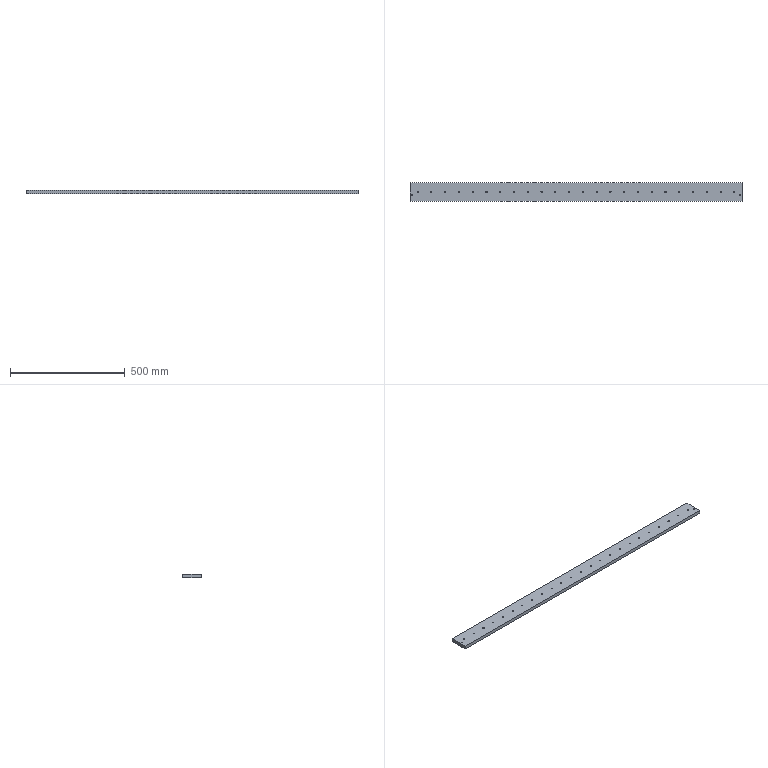Part | NX | 1 solid | 36 faces | box 1446 x 80 x 15 mm | volume 1727896 mm3 | cylinder 26 | plane 6 | cone 4 | commonest cylinder face diameters 5 x24 3 x2
STEP:
#1=CARTESIAN_POINT('',(723.,-40.,0.));
#2=VERTEX_POINT('',#1);
#3=CARTESIAN_POINT('',(723.,40.,0.));
#4=VERTEX_POINT('',#3);
#5=CARTESIAN_POINT('',(723.,-40.,0.));
#6=DIRECTION('',(0.,1.,0.));
#7=VECTOR('',#6,1000.);
#8=LINE('',#5,#7);
#9=EDGE_CURVE('',#2,#4,#8,.T.);
#10=ORIENTED_EDGE('',*,*,#9,.T.);
#11=CARTESIAN_POINT('',(723.,40.,15.));
#12=VERTEX_POINT('',#11);
#13=CARTESIAN_POINT('',(723.,40.,15.));
#14=DIRECTION('',(0.,0.,-1.));
#15=VECTOR('',#14,1000.);
#16=LINE('',#13,#15);
#17=EDGE_CURVE('',#12,#4,#16,.T.);
#18=ORIENTED_EDGE('',*,*,#17,.F.);
#19=CARTESIAN_POINT('',(723.,-40.,15.));
#20=VERTEX_POINT('',#19);
#21=CARTESIAN_POINT('',(723.,-40.,15.));
#22=DIRECTION('',(0.,1.,0.));
#23=VECTOR('',#22,1000.);
#24=LINE('',#21,#23);
#25=EDGE_CURVE('',#20,#12,#24,.T.);
#26=ORIENTED_EDGE('',*,*,#25,.F.);
#27=CARTESIAN_POINT('',(723.,-40.,15.));
#28=DIRECTION('',(0.,0.,-1.));
#29=VECTOR('',#28,1000.);
#30=LINE('',#27,#29);
#31=EDGE_CURVE('',#20,#2,#30,.T.);
#32=ORIENTED_EDGE('',*,*,#31,.T.);
#33=EDGE_LOOP('',(#10,#18,#26,#32));
#34=FACE_BOUND('',#33,.T.);
#35=CARTESIAN_POINT('',(723.,-40.,15.));
#36=DIRECTION('',(-1.,0.,0.));
#37=DIRECTION('',(0.,0.,1.));
#38=AXIS2_PLACEMENT_3D('',#35,#36,#37);
#39=PLANE('',#38);
#40=ADVANCED_FACE('',(#34),#39,.F.);
#41=CARTESIAN_POINT('',(-723.,40.,0.));
#42=VERTEX_POINT('',#41);
#43=CARTESIAN_POINT('',(-723.,40.,0.));
#44=DIRECTION('',(-1.,0.,0.));
#45=VECTOR('',#44,1000.);
#46=LINE('',#43,#45);
#47=EDGE_CURVE('',#4,#42,#46,.T.);
#48=ORIENTED_EDGE('',*,*,#47,.T.);
#49=CARTESIAN_POINT('',(-723.,40.,15.));
#50=VERTEX_POINT('',#49);
#51=CARTESIAN_POINT('',(-723.,40.,15.));
#52=DIRECTION('',(0.,0.,-1.));
#53=VECTOR('',#52,1000.);
#54=LINE('',#51,#53);
#55=EDGE_CURVE('',#50,#42,#54,.T.);
#56=ORIENTED_EDGE('',*,*,#55,.F.);
#57=CARTESIAN_POINT('',(-723.,40.,15.));
#58=DIRECTION('',(-1.,0.,0.));
#59=VECTOR('',#58,1000.);
#60=LINE('',#57,#59);
#61=EDGE_CURVE('',#12,#50,#60,.T.);
#62=ORIENTED_EDGE('',*,*,#61,.F.);
#63=ORIENTED_EDGE('',*,*,#17,.T.);
#64=EDGE_LOOP('',(#48,#56,#62,#63));
#65=FACE_BOUND('',#64,.T.);
#66=CARTESIAN_POINT('',(-723.,40.,15.));
#67=DIRECTION('',(0.,-1.,0.));
#68=DIRECTION('',(0.,0.,-1.));
#69=AXIS2_PLACEMENT_3D('',#66,#67,#68);
#70=PLANE('',#69);
#71=ADVANCED_FACE('',(#65),#70,.F.);
#72=CARTESIAN_POINT('',(-723.,-40.,0.));
#73=VERTEX_POINT('',#72);
#74=CARTESIAN_POINT('',(-723.,-40.,0.));
#75=DIRECTION('',(0.,-1.,0.));
#76=VECTOR('',#75,1000.);
#77=LINE('',#74,#76);
#78=EDGE_CURVE('',#42,#73,#77,.T.);
#79=ORIENTED_EDGE('',*,*,#78,.T.);
#80=CARTESIAN_POINT('',(-723.,-40.,15.));
#81=VERTEX_POINT('',#80);
#82=CARTESIAN_POINT('',(-723.,-40.,15.));
#83=DIRECTION('',(0.,0.,-1.));
#84=VECTOR('',#83,1000.);
#85=LINE('',#82,#84);
#86=EDGE_CURVE('',#81,#73,#85,.T.);
#87=ORIENTED_EDGE('',*,*,#86,.F.);
#88=CARTESIAN_POINT('',(-723.,-40.,15.));
#89=DIRECTION('',(0.,-1.,0.));
#90=VECTOR('',#89,1000.);
#91=LINE('',#88,#90);
#92=EDGE_CURVE('',#50,#81,#91,.T.);
#93=ORIENTED_EDGE('',*,*,#92,.F.);
#94=ORIENTED_EDGE('',*,*,#55,.T.);
#95=EDGE_LOOP('',(#79,#87,#93,#94));
#96=FACE_BOUND('',#95,.T.);
#97=CARTESIAN_POINT('',(-723.,-40.,15.));
#98=DIRECTION('',(1.,0.,0.));
#99=DIRECTION('',(0.,0.,-1.));
#100=AXIS2_PLACEMENT_3D('',#97,#98,#99);
#101=PLANE('',#100);
#102=ADVANCED_FACE('',(#96),#101,.F.);
#103=CARTESIAN_POINT('',(-723.,-40.,0.));
#104=DIRECTION('',(1.,0.,0.));
#105=VECTOR('',#104,1000.);
#106=LINE('',#103,#105);
#107=EDGE_CURVE('',#73,#2,#106,.T.);
#108=ORIENTED_EDGE('',*,*,#107,.T.);
#109=ORIENTED_EDGE('',*,*,#31,.F.);
#110=CARTESIAN_POINT('',(-723.,-40.,15.));
#111=DIRECTION('',(1.,0.,0.));
#112=VECTOR('',#111,1000.);
#113=LINE('',#110,#112);
#114=EDGE_CURVE('',#81,#20,#113,.T.);
#115=ORIENTED_EDGE('',*,*,#114,.F.);
#116=ORIENTED_EDGE('',*,*,#86,.T.);
#117=EDGE_LOOP('',(#108,#109,#115,#116));
#118=FACE_BOUND('',#117,.T.);
#119=CARTESIAN_POINT('',(-723.,-40.,15.));
#120=DIRECTION('',(0.,1.,0.));
#121=DIRECTION('',(0.,0.,1.));
#122=AXIS2_PLACEMENT_3D('',#119,#120,#121);
#123=PLANE('',#122);
#124=ADVANCED_FACE('',(#118),#123,.F.);
#125=CARTESIAN_POINT('',(710.5,-13.,15.));
#126=VERTEX_POINT('',#125);
#127=CARTESIAN_POINT('',(713.,-13.,15.));
#128=DIRECTION('',(0.,0.,-1.));
#129=DIRECTION('',(-1.,0.,0.));
#130=AXIS2_PLACEMENT_3D('',#127,#128,#129);
#131=CIRCLE('',#130,2.5);
#132=EDGE_CURVE('',#126,#126,#131,.T.);
#133=ORIENTED_EDGE('',*,*,#132,.T.);
#134=EDGE_LOOP('',(#133));
#135=FACE_BOUND('',#134,.T.);
#136=CARTESIAN_POINT('',(-715.5,-13.,15.));
#137=VERTEX_POINT('',#136);
#138=CARTESIAN_POINT('',(-713.,-13.,15.));
#139=DIRECTION('',(0.,0.,-1.));
#140=DIRECTION('',(-1.,0.,0.));
#141=AXIS2_PLACEMENT_3D('',#138,#139,#140);
#142=CIRCLE('',#141,2.5);
#143=EDGE_CURVE('',#137,#137,#142,.T.);
#144=ORIENTED_EDGE('',*,*,#143,.T.);
#145=EDGE_LOOP('',(#144));
#146=FACE_BOUND('',#145,.T.);
#147=CARTESIAN_POINT('',(-627.5,0.,15.));
#148=VERTEX_POINT('',#147);
#149=CARTESIAN_POINT('',(-630.,0.,15.));
#150=DIRECTION('',(0.,0.,1.));
#151=DIRECTION('',(1.,0.,0.));
#152=AXIS2_PLACEMENT_3D('',#149,#150,#151);
#153=CIRCLE('',#152,2.5);
#154=EDGE_CURVE('',#148,#148,#153,.T.);
#155=ORIENTED_EDGE('',*,*,#154,.F.);
#156=EDGE_LOOP('',(#155));
#157=FACE_BOUND('',#156,.T.);
#158=CARTESIAN_POINT('',(-687.5,0.,15.));
#159=VERTEX_POINT('',#158);
#160=CARTESIAN_POINT('',(-690.,0.,15.));
#161=DIRECTION('',(0.,0.,1.));
#162=DIRECTION('',(1.,0.,0.));
#163=AXIS2_PLACEMENT_3D('',#160,#161,#162);
#164=CIRCLE('',#163,2.5);
#165=EDGE_CURVE('',#159,#159,#164,.T.);
#166=ORIENTED_EDGE('',*,*,#165,.F.);
#167=EDGE_LOOP('',(#166));
#168=FACE_BOUND('',#167,.T.);
#169=ORIENTED_EDGE('',*,*,#25,.T.);
#170=ORIENTED_EDGE('',*,*,#61,.T.);
#171=ORIENTED_EDGE('',*,*,#92,.T.);
#172=ORIENTED_EDGE('',*,*,#114,.T.);
#173=EDGE_LOOP('',(#169,#170,#171,#172));
#174=FACE_BOUND('',#173,.T.);
#175=CARTESIAN_POINT('',(-567.5,0.,15.));
#176=VERTEX_POINT('',#175);
#177=CARTESIAN_POINT('',(-570.,0.,15.));
#178=DIRECTION('',(0.,0.,1.));
#179=DIRECTION('',(1.,0.,0.));
#180=AXIS2_PLACEMENT_3D('',#177,#178,#179);
#181=CIRCLE('',#180,2.5);
#182=EDGE_CURVE('',#176,#176,#181,.T.);
#183=ORIENTED_EDGE('',*,*,#182,.F.);
#184=EDGE_LOOP('',(#183));
#185=FACE_BOUND('',#184,.T.);
#186=CARTESIAN_POINT('',(-507.5,0.,15.));
#187=VERTEX_POINT('',#186);
#188=CARTESIAN_POINT('',(-510.,0.,15.));
#189=DIRECTION('',(0.,0.,1.));
#190=DIRECTION('',(1.,0.,0.));
#191=AXIS2_PLACEMENT_3D('',#188,#189,#190);
#192=CIRCLE('',#191,2.5);
#193=EDGE_CURVE('',#187,#187,#192,.T.);
#194=ORIENTED_EDGE('',*,*,#193,.F.);
#195=EDGE_LOOP('',(#194));
#196=FACE_BOUND('',#195,.T.);
#197=CARTESIAN_POINT('',(-447.5,0.,15.));
#198=VERTEX_POINT('',#197);
#199=CARTESIAN_POINT('',(-450.,0.,15.));
#200=DIRECTION('',(0.,0.,1.));
#201=DIRECTION('',(1.,0.,0.));
#202=AXIS2_PLACEMENT_3D('',#199,#200,#201);
#203=CIRCLE('',#202,2.5);
#204=EDGE_CURVE('',#198,#198,#203,.T.);
#205=ORIENTED_EDGE('',*,*,#204,.F.);
#206=EDGE_LOOP('',(#205));
#207=FACE_BOUND('',#206,.T.);
#208=CARTESIAN_POINT('',(-387.5,0.,15.));
#209=VERTEX_POINT('',#208);
#210=CARTESIAN_POINT('',(-390.,0.,15.));
#211=DIRECTION('',(0.,0.,1.));
#212=DIRECTION('',(1.,0.,0.));
#213=AXIS2_PLACEMENT_3D('',#210,#211,#212);
#214=CIRCLE('',#213,2.5);
#215=EDGE_CURVE('',#209,#209,#214,.T.);
#216=ORIENTED_EDGE('',*,*,#215,.F.);
#217=EDGE_LOOP('',(#216));
#218=FACE_BOUND('',#217,.T.);
#219=CARTESIAN_POINT('',(-327.5,0.,15.));
#220=VERTEX_POINT('',#219);
#221=CARTESIAN_POINT('',(-330.,0.,15.));
#222=DIRECTION('',(0.,0.,1.));
#223=DIRECTION('',(1.,0.,0.));
#224=AXIS2_PLACEMENT_3D('',#221,#222,#223);
#225=CIRCLE('',#224,2.5);
#226=EDGE_CURVE('',#220,#220,#225,.T.);
#227=ORIENTED_EDGE('',*,*,#226,.F.);
#228=EDGE_LOOP('',(#227));
#229=FACE_BOUND('',#228,.T.);
#230=CARTESIAN_POINT('',(-267.5,0.,15.));
#231=VERTEX_POINT('',#230);
#232=CARTESIAN_POINT('',(-270.,0.,15.));
#233=DIRECTION('',(0.,0.,1.));
#234=DIRECTION('',(1.,0.,0.));
#235=AXIS2_PLACEMENT_3D('',#232,#233,#234);
#236=CIRCLE('',#235,2.5);
#237=EDGE_CURVE('',#231,#231,#236,.T.);
#238=ORIENTED_EDGE('',*,*,#237,.F.);
#239=EDGE_LOOP('',(#238));
#240=FACE_BOUND('',#239,.T.);
#241=CARTESIAN_POINT('',(-207.5,0.,15.));
#242=VERTEX_POINT('',#241);
#243=CARTESIAN_POINT('',(-210.,0.,15.));
#244=DIRECTION('',(0.,0.,1.));
#245=DIRECTION('',(1.,0.,0.));
#246=AXIS2_PLACEMENT_3D('',#243,#244,#245);
#247=CIRCLE('',#246,2.5);
#248=EDGE_CURVE('',#242,#242,#247,.T.);
#249=ORIENTED_EDGE('',*,*,#248,.F.);
#250=EDGE_LOOP('',(#249));
#251=FACE_BOUND('',#250,.T.);
#252=CARTESIAN_POINT('',(-147.5,0.,15.));
#253=VERTEX_POINT('',#252);
#254=CARTESIAN_POINT('',(-150.,0.,15.));
#255=DIRECTION('',(0.,0.,1.));
#256=DIRECTION('',(1.,0.,0.));
#257=AXIS2_PLACEMENT_3D('',#254,#255,#256);
#258=CIRCLE('',#257,2.5);
#259=EDGE_CURVE('',#253,#253,#258,.T.);
#260=ORIENTED_EDGE('',*,*,#259,.F.);
#261=EDGE_LOOP('',(#260));
#262=FACE_BOUND('',#261,.T.);
#263=CARTESIAN_POINT('',(-87.5,0.,15.));
#264=VERTEX_POINT('',#263);
#265=CARTESIAN_POINT('',(-90.,0.,15.));
#266=DIRECTION('',(0.,0.,1.));
#267=DIRECTION('',(1.,0.,0.));
#268=AXIS2_PLACEMENT_3D('',#265,#266,#267);
#269=CIRCLE('',#268,2.5);
#270=EDGE_CURVE('',#264,#264,#269,.T.);
#271=ORIENTED_EDGE('',*,*,#270,.F.);
#272=EDGE_LOOP('',(#271));
#273=FACE_BOUND('',#272,.T.);
#274=CARTESIAN_POINT('',(-27.5,0.,15.));
#275=VERTEX_POINT('',#274);
#276=CARTESIAN_POINT('',(-30.,0.,15.));
#277=DIRECTION('',(0.,0.,1.));
#278=DIRECTION('',(1.,0.,0.));
#279=AXIS2_PLACEMENT_3D('',#276,#277,#278);
#280=CIRCLE('',#279,2.5);
#281=EDGE_CURVE('',#275,#275,#280,.T.);
#282=ORIENTED_EDGE('',*,*,#281,.F.);
#283=EDGE_LOOP('',(#282));
#284=FACE_BOUND('',#283,.T.);
#285=CARTESIAN_POINT('',(32.5,0.,15.));
#286=VERTEX_POINT('',#285);
#287=CARTESIAN_POINT('',(30.,0.,15.));
#288=DIRECTION('',(0.,0.,1.));
#289=DIRECTION('',(1.,0.,0.));
#290=AXIS2_PLACEMENT_3D('',#287,#288,#289);
#291=CIRCLE('',#290,2.5);
#292=EDGE_CURVE('',#286,#286,#291,.T.);
#293=ORIENTED_EDGE('',*,*,#292,.F.);
#294=EDGE_LOOP('',(#293));
#295=FACE_BOUND('',#294,.T.);
#296=CARTESIAN_POINT('',(92.5,0.,15.));
#297=VERTEX_POINT('',#296);
#298=CARTESIAN_POINT('',(90.,0.,15.));
#299=DIRECTION('',(0.,0.,1.));
#300=DIRECTION('',(1.,0.,0.));
#301=AXIS2_PLACEMENT_3D('',#298,#299,#300);
#302=CIRCLE('',#301,2.5);
#303=EDGE_CURVE('',#297,#297,#302,.T.);
#304=ORIENTED_EDGE('',*,*,#303,.F.);
#305=EDGE_LOOP('',(#304));
#306=FACE_BOUND('',#305,.T.);
#307=CARTESIAN_POINT('',(152.5,0.,15.));
#308=VERTEX_POINT('',#307);
#309=CARTESIAN_POINT('',(150.,0.,15.));
#310=DIRECTION('',(0.,0.,1.));
#311=DIRECTION('',(1.,0.,0.));
#312=AXIS2_PLACEMENT_3D('',#309,#310,#311);
#313=CIRCLE('',#312,2.5);
#314=EDGE_CURVE('',#308,#308,#313,.T.);
#315=ORIENTED_EDGE('',*,*,#314,.F.);
#316=EDGE_LOOP('',(#315));
#317=FACE_BOUND('',#316,.T.);
#318=CARTESIAN_POINT('',(212.5,0.,15.));
#319=VERTEX_POINT('',#318);
#320=CARTESIAN_POINT('',(210.,0.,15.));
#321=DIRECTION('',(0.,0.,1.));
#322=DIRECTION('',(1.,0.,0.));
#323=AXIS2_PLACEMENT_3D('',#320,#321,#322);
#324=CIRCLE('',#323,2.5);
#325=EDGE_CURVE('',#319,#319,#324,.T.);
#326=ORIENTED_EDGE('',*,*,#325,.F.);
#327=EDGE_LOOP('',(#326));
#328=FACE_BOUND('',#327,.T.);
#329=CARTESIAN_POINT('',(272.5,0.,15.));
#330=VERTEX_POINT('',#329);
#331=CARTESIAN_POINT('',(270.,0.,15.));
#332=DIRECTION('',(0.,0.,1.));
#333=DIRECTION('',(1.,0.,0.));
#334=AXIS2_PLACEMENT_3D('',#331,#332,#333);
#335=CIRCLE('',#334,2.5);
#336=EDGE_CURVE('',#330,#330,#335,.T.);
#337=ORIENTED_EDGE('',*,*,#336,.F.);
#338=EDGE_LOOP('',(#337));
#339=FACE_BOUND('',#338,.T.);
#340=CARTESIAN_POINT('',(332.5,0.,15.));
#341=VERTEX_POINT('',#340);
#342=CARTESIAN_POINT('',(330.,0.,15.));
#343=DIRECTION('',(0.,0.,1.));
#344=DIRECTION('',(1.,0.,0.));
#345=AXIS2_PLACEMENT_3D('',#342,#343,#344);
#346=CIRCLE('',#345,2.5);
#347=EDGE_CURVE('',#341,#341,#346,.T.);
#348=ORIENTED_EDGE('',*,*,#347,.F.);
#349=EDGE_LOOP('',(#348));
#350=FACE_BOUND('',#349,.T.);
#351=CARTESIAN_POINT('',(392.5,0.,15.));
#352=VERTEX_POINT('',#351);
#353=CARTESIAN_POINT('',(390.,0.,15.));
#354=DIRECTION('',(0.,0.,1.));
#355=DIRECTION('',(1.,0.,0.));
#356=AXIS2_PLACEMENT_3D('',#353,#354,#355);
#357=CIRCLE('',#356,2.5);
#358=EDGE_CURVE('',#352,#352,#357,.T.);
#359=ORIENTED_EDGE('',*,*,#358,.F.);
#360=EDGE_LOOP('',(#359));
#361=FACE_BOUND('',#360,.T.);
#362=CARTESIAN_POINT('',(452.5,0.,15.));
#363=VERTEX_POINT('',#362);
#364=CARTESIAN_POINT('',(450.,0.,15.));
#365=DIRECTION('',(0.,0.,1.));
#366=DIRECTION('',(1.,0.,0.));
#367=AXIS2_PLACEMENT_3D('',#364,#365,#366);
#368=CIRCLE('',#367,2.5);
#369=EDGE_CURVE('',#363,#363,#368,.T.);
#370=ORIENTED_EDGE('',*,*,#369,.F.);
#371=EDGE_LOOP('',(#370));
#372=FACE_BOUND('',#371,.T.);
#373=CARTESIAN_POINT('',(512.5,0.,15.));
#374=VERTEX_POINT('',#373);
#375=CARTESIAN_POINT('',(510.,0.,15.));
#376=DIRECTION('',(0.,0.,1.));
#377=DIRECTION('',(1.,0.,0.));
#378=AXIS2_PLACEMENT_3D('',#375,#376,#377);
#379=CIRCLE('',#378,2.5);
#380=EDGE_CURVE('',#374,#374,#379,.T.);
#381=ORIENTED_EDGE('',*,*,#380,.F.);
#382=EDGE_LOOP('',(#381));
#383=FACE_BOUND('',#382,.T.);
#384=CARTESIAN_POINT('',(572.5,0.,15.));
#385=VERTEX_POINT('',#384);
#386=CARTESIAN_POINT('',(570.,0.,15.));
#387=DIRECTION('',(0.,0.,1.));
#388=DIRECTION('',(1.,0.,0.));
#389=AXIS2_PLACEMENT_3D('',#386,#387,#388);
#390=CIRCLE('',#389,2.5);
#391=EDGE_CURVE('',#385,#385,#390,.T.);
#392=ORIENTED_EDGE('',*,*,#391,.F.);
#393=EDGE_LOOP('',(#392));
#394=FACE_BOUND('',#393,.T.);
#395=CARTESIAN_POINT('',(632.5,0.,15.));
#396=VERTEX_POINT('',#395);
#397=CARTESIAN_POINT('',(630.,0.,15.));
#398=DIRECTION('',(0.,0.,1.));
#399=DIRECTION('',(1.,0.,0.));
#400=AXIS2_PLACEMENT_3D('',#397,#398,#399);
#401=CIRCLE('',#400,2.5);
#402=EDGE_CURVE('',#396,#396,#401,.T.);
#403=ORIENTED_EDGE('',*,*,#402,.F.);
#404=EDGE_LOOP('',(#403));
#405=FACE_BOUND('',#404,.T.);
#406=CARTESIAN_POINT('',(692.5,0.,15.));
#407=VERTEX_POINT('',#406);
#408=CARTESIAN_POINT('',(690.,0.,15.));
#409=DIRECTION('',(0.,0.,1.));
#410=DIRECTION('',(1.,0.,0.));
#411=AXIS2_PLACEMENT_3D('',#408,#409,#410);
#412=CIRCLE('',#411,2.5);
#413=EDGE_CURVE('',#407,#407,#412,.T.);
#414=ORIENTED_EDGE('',*,*,#413,.F.);
#415=EDGE_LOOP('',(#414));
#416=FACE_BOUND('',#415,.T.);
#417=CARTESIAN_POINT('',(0.,0.,15.));
#418=DIRECTION('',(0.,0.,-1.));
#419=DIRECTION('',(-1.,0.,0.));
#420=AXIS2_PLACEMENT_3D('',#417,#418,#419);
#421=PLANE('',#420);
#422=ADVANCED_FACE('',(#135,#146,#157,#168,#174,#185,#196,#207,#218,#229,#240,#251,#262,#273,#284,#295,#306,#317,#328,#339,#350,#361,#372,#383,#394,#405,#416),#421,.F.);
#423=CARTESIAN_POINT('',(710.5,-13.,0.));
#424=VERTEX_POINT('',#423);
#425=CARTESIAN_POINT('',(713.,-13.,0.));
#426=DIRECTION('',(0.,0.,-1.));
#427=DIRECTION('',(-1.,0.,0.));
#428=AXIS2_PLACEMENT_3D('',#425,#426,#427);
#429=CIRCLE('',#428,2.5);
#430=EDGE_CURVE('',#424,#424,#429,.F.);
#431=ORIENTED_EDGE('',*,*,#430,.T.);
#432=EDGE_LOOP('',(#431));
#433=FACE_BOUND('',#432,.T.);
#434=CARTESIAN_POINT('',(-715.5,-13.,0.));
#435=VERTEX_POINT('',#434);
#436=CARTESIAN_POINT('',(-713.,-13.,0.));
#437=DIRECTION('',(0.,0.,-1.));
#438=DIRECTION('',(-1.,0.,0.));
#439=AXIS2_PLACEMENT_3D('',#436,#437,#438);
#440=CIRCLE('',#439,2.5);
#441=EDGE_CURVE('',#435,#435,#440,.F.);
#442=ORIENTED_EDGE('',*,*,#441,.T.);
#443=EDGE_LOOP('',(#442));
#444=FACE_BOUND('',#443,.T.);
#445=CARTESIAN_POINT('',(-632.5,0.,0.));
#446=VERTEX_POINT('',#445);
#447=CARTESIAN_POINT('',(-630.,0.,0.));
#448=DIRECTION('',(0.,0.,-1.));
#449=DIRECTION('',(-1.,0.,0.));
#450=AXIS2_PLACEMENT_3D('',#447,#448,#449);
#451=CIRCLE('',#450,2.5);
#452=EDGE_CURVE('',#446,#446,#451,.T.);
#453=ORIENTED_EDGE('',*,*,#452,.F.);
#454=EDGE_LOOP('',(#453));
#455=FACE_BOUND('',#454,.T.);
#456=CARTESIAN_POINT('',(-692.5,0.,0.));
#457=VERTEX_POINT('',#456);
#458=CARTESIAN_POINT('',(-690.,0.,0.));
#459=DIRECTION('',(0.,0.,-1.));
#460=DIRECTION('',(-1.,0.,0.));
#461=AXIS2_PLACEMENT_3D('',#458,#459,#460);
#462=CIRCLE('',#461,2.5);
#463=EDGE_CURVE('',#457,#457,#462,.T.);
#464=ORIENTED_EDGE('',*,*,#463,.F.);
#465=EDGE_LOOP('',(#464));
#466=FACE_BOUND('',#465,.T.);
#467=ORIENTED_EDGE('',*,*,#9,.F.);
#468=ORIENTED_EDGE('',*,*,#107,.F.);
#469=ORIENTED_EDGE('',*,*,#78,.F.);
#470=ORIENTED_EDGE('',*,*,#47,.F.);
#471=EDGE_LOOP('',(#467,#468,#469,#470));
#472=FACE_BOUND('',#471,.T.);
#473=CARTESIAN_POINT('',(-572.5,0.,0.));
#474=VERTEX_POINT('',#473);
#475=CARTESIAN_POINT('',(-570.,0.,0.));
#476=DIRECTION('',(0.,0.,-1.));
#477=DIRECTION('',(-1.,0.,0.));
#478=AXIS2_PLACEMENT_3D('',#475,#476,#477);
#479=CIRCLE('',#478,2.5);
#480=EDGE_CURVE('',#474,#474,#479,.T.);
#481=ORIENTED_EDGE('',*,*,#480,.F.);
#482=EDGE_LOOP('',(#481));
#483=FACE_BOUND('',#482,.T.);
#484=CARTESIAN_POINT('',(-512.5,0.,0.));
#485=VERTEX_POINT('',#484);
#486=CARTESIAN_POINT('',(-510.,0.,0.));
#487=DIRECTION('',(0.,0.,-1.));
#488=DIRECTION('',(-1.,0.,0.));
#489=AXIS2_PLACEMENT_3D('',#486,#487,#488);
#490=CIRCLE('',#489,2.5);
#491=EDGE_CURVE('',#485,#485,#490,.T.);
#492=ORIENTED_EDGE('',*,*,#491,.F.);
#493=EDGE_LOOP('',(#492));
#494=FACE_BOUND('',#493,.T.);
#495=CARTESIAN_POINT('',(-452.5,0.,0.));
#496=VERTEX_POINT('',#495);
#497=CARTESIAN_POINT('',(-450.,0.,0.));
#498=DIRECTION('',(0.,0.,-1.));
#499=DIRECTION('',(-1.,0.,0.));
#500=AXIS2_PLACEMENT_3D('',#497,#498,#499);
#501=CIRCLE('',#500,2.5);
#502=EDGE_CURVE('',#496,#496,#501,.T.);
#503=ORIENTED_EDGE('',*,*,#502,.F.);
#504=EDGE_LOOP('',(#503));
#505=FACE_BOUND('',#504,.T.);
#506=CARTESIAN_POINT('',(-392.5,0.,0.));
#507=VERTEX_POINT('',#506);
#508=CARTESIAN_POINT('',(-390.,0.,0.));
#509=DIRECTION('',(0.,0.,-1.));
#510=DIRECTION('',(-1.,0.,0.));
#511=AXIS2_PLACEMENT_3D('',#508,#509,#510);
#512=CIRCLE('',#511,2.5);
#513=EDGE_CURVE('',#507,#507,#512,.T.);
#514=ORIENTED_EDGE('',*,*,#513,.F.);
#515=EDGE_LOOP('',(#514));
#516=FACE_BOUND('',#515,.T.);
#517=CARTESIAN_POINT('',(-332.5,0.,0.));
#518=VERTEX_POINT('',#517);
#519=CARTESIAN_POINT('',(-330.,0.,0.));
#520=DIRECTION('',(0.,0.,-1.));
#521=DIRECTION('',(-1.,0.,0.));
#522=AXIS2_PLACEMENT_3D('',#519,#520,#521);
#523=CIRCLE('',#522,2.5);
#524=EDGE_CURVE('',#518,#518,#523,.T.);
#525=ORIENTED_EDGE('',*,*,#524,.F.);
#526=EDGE_LOOP('',(#525));
#527=FACE_BOUND('',#526,.T.);
#528=CARTESIAN_POINT('',(-272.5,0.,0.));
#529=VERTEX_POINT('',#528);
#530=CARTESIAN_POINT('',(-270.,0.,0.));
#531=DIRECTION('',(0.,0.,-1.));
#532=DIRECTION('',(-1.,0.,0.));
#533=AXIS2_PLACEMENT_3D('',#530,#531,#532);
#534=CIRCLE('',#533,2.5);
#535=EDGE_CURVE('',#529,#529,#534,.T.);
#536=ORIENTED_EDGE('',*,*,#535,.F.);
#537=EDGE_LOOP('',(#536));
#538=FACE_BOUND('',#537,.T.);
#539=CARTESIAN_POINT('',(-212.5,0.,0.));
#540=VERTEX_POINT('',#539);
#541=CARTESIAN_POINT('',(-210.,0.,0.));
#542=DIRECTION('',(0.,0.,-1.));
#543=DIRECTION('',(-1.,0.,0.));
#544=AXIS2_PLACEMENT_3D('',#541,#542,#543);
#545=CIRCLE('',#544,2.5);
#546=EDGE_CURVE('',#540,#540,#545,.T.);
#547=ORIENTED_EDGE('',*,*,#546,.F.);
#548=EDGE_LOOP('',(#547));
#549=FACE_BOUND('',#548,.T.);
#550=CARTESIAN_POINT('',(-152.5,0.,0.));
#551=VERTEX_POINT('',#550);
#552=CARTESIAN_POINT('',(-150.,0.,0.));
#553=DIRECTION('',(0.,0.,-1.));
#554=DIRECTION('',(-1.,0.,0.));
#555=AXIS2_PLACEMENT_3D('',#552,#553,#554);
#556=CIRCLE('',#555,2.5);
#557=EDGE_CURVE('',#551,#551,#556,.T.);
#558=ORIENTED_EDGE('',*,*,#557,.F.);
#559=EDGE_LOOP('',(#558));
#560=FACE_BOUND('',#559,.T.);
#561=CARTESIAN_POINT('',(-92.5,0.,0.));
#562=VERTEX_POINT('',#561);
#563=CARTESIAN_POINT('',(-90.,0.,0.));
#564=DIRECTION('',(0.,0.,-1.));
#565=DIRECTION('',(-1.,0.,0.));
#566=AXIS2_PLACEMENT_3D('',#563,#564,#565);
#567=CIRCLE('',#566,2.5);
#568=EDGE_CURVE('',#562,#562,#567,.T.);
#569=ORIENTED_EDGE('',*,*,#568,.F.);
#570=EDGE_LOOP('',(#569));
#571=FACE_BOUND('',#570,.T.);
#572=CARTESIAN_POINT('',(-32.5,0.,0.));
#573=VERTEX_POINT('',#572);
#574=CARTESIAN_POINT('',(-30.,0.,0.));
#575=DIRECTION('',(0.,0.,-1.));
#576=DIRECTION('',(-1.,0.,0.));
#577=AXIS2_PLACEMENT_3D('',#574,#575,#576);
#578=CIRCLE('',#577,2.5);
#579=EDGE_CURVE('',#573,#573,#578,.T.);
#580=ORIENTED_EDGE('',*,*,#579,.F.);
#581=EDGE_LOOP('',(#580));
#582=FACE_BOUND('',#581,.T.);
#583=CARTESIAN_POINT('',(27.5,0.,0.));
#584=VERTEX_POINT('',#583);
#585=CARTESIAN_POINT('',(30.,0.,0.));
#586=DIRECTION('',(0.,0.,-1.));
#587=DIRECTION('',(-1.,0.,0.));
#588=AXIS2_PLACEMENT_3D('',#585,#586,#587);
#589=CIRCLE('',#588,2.5);
#590=EDGE_CURVE('',#584,#584,#589,.T.);
#591=ORIENTED_EDGE('',*,*,#590,.F.);
#592=EDGE_LOOP('',(#591));
#593=FACE_BOUND('',#592,.T.);
#594=CARTESIAN_POINT('',(87.5,0.,0.));
#595=VERTEX_POINT('',#594);
#596=CARTESIAN_POINT('',(90.,0.,0.));
#597=DIRECTION('',(0.,0.,-1.));
#598=DIRECTION('',(-1.,0.,0.));
#599=AXIS2_PLACEMENT_3D('',#596,#597,#598);
#600=CIRCLE('',#599,2.5);
#601=EDGE_CURVE('',#595,#595,#600,.T.);
#602=ORIENTED_EDGE('',*,*,#601,.F.);
#603=EDGE_LOOP('',(#602));
#604=FACE_BOUND('',#603,.T.);
#605=CARTESIAN_POINT('',(147.5,0.,0.));
#606=VERTEX_POINT('',#605);
#607=CARTESIAN_POINT('',(150.,0.,0.));
#608=DIRECTION('',(0.,0.,-1.));
#609=DIRECTION('',(-1.,0.,0.));
#610=AXIS2_PLACEMENT_3D('',#607,#608,#609);
#611=CIRCLE('',#610,2.5);
#612=EDGE_CURVE('',#606,#606,#611,.T.);
#613=ORIENTED_EDGE('',*,*,#612,.F.);
#614=EDGE_LOOP('',(#613));
#615=FACE_BOUND('',#614,.T.);
#616=CARTESIAN_POINT('',(207.5,0.,0.));
#617=VERTEX_POINT('',#616);
#618=CARTESIAN_POINT('',(210.,0.,0.));
#619=DIRECTION('',(0.,0.,-1.));
#620=DIRECTION('',(-1.,0.,0.));
#621=AXIS2_PLACEMENT_3D('',#618,#619,#620);
#622=CIRCLE('',#621,2.5);
#623=EDGE_CURVE('',#617,#617,#622,.T.);
#624=ORIENTED_EDGE('',*,*,#623,.F.);
#625=EDGE_LOOP('',(#624));
#626=FACE_BOUND('',#625,.T.);
#627=CARTESIAN_POINT('',(267.5,0.,0.));
#628=VERTEX_POINT('',#627);
#629=CARTESIAN_POINT('',(270.,0.,0.));
#630=DIRECTION('',(0.,0.,-1.));
#631=DIRECTION('',(-1.,0.,0.));
#632=AXIS2_PLACEMENT_3D('',#629,#630,#631);
#633=CIRCLE('',#632,2.5);
#634=EDGE_CURVE('',#628,#628,#633,.T.);
#635=ORIENTED_EDGE('',*,*,#634,.F.);
#636=EDGE_LOOP('',(#635));
#637=FACE_BOUND('',#636,.T.);
#638=CARTESIAN_POINT('',(327.5,0.,0.));
#639=VERTEX_POINT('',#638);
#640=CARTESIAN_POINT('',(330.,0.,0.));
#641=DIRECTION('',(0.,0.,-1.));
#642=DIRECTION('',(-1.,0.,0.));
#643=AXIS2_PLACEMENT_3D('',#640,#641,#642);
#644=CIRCLE('',#643,2.5);
#645=EDGE_CURVE('',#639,#639,#644,.T.);
#646=ORIENTED_EDGE('',*,*,#645,.F.);
#647=EDGE_LOOP('',(#646));
#648=FACE_BOUND('',#647,.T.);
#649=CARTESIAN_POINT('',(387.5,0.,0.));
#650=VERTEX_POINT('',#649);
#651=CARTESIAN_POINT('',(390.,0.,0.));
#652=DIRECTION('',(0.,0.,-1.));
#653=DIRECTION('',(-1.,0.,0.));
#654=AXIS2_PLACEMENT_3D('',#651,#652,#653);
#655=CIRCLE('',#654,2.5);
#656=EDGE_CURVE('',#650,#650,#655,.T.);
#657=ORIENTED_EDGE('',*,*,#656,.F.);
#658=EDGE_LOOP('',(#657));
#659=FACE_BOUND('',#658,.T.);
#660=CARTESIAN_POINT('',(447.5,0.,0.));
#661=VERTEX_POINT('',#660);
#662=CARTESIAN_POINT('',(450.,0.,0.));
#663=DIRECTION('',(0.,0.,-1.));
#664=DIRECTION('',(-1.,0.,0.));
#665=AXIS2_PLACEMENT_3D('',#662,#663,#664);
#666=CIRCLE('',#665,2.5);
#667=EDGE_CURVE('',#661,#661,#666,.T.);
#668=ORIENTED_EDGE('',*,*,#667,.F.);
#669=EDGE_LOOP('',(#668));
#670=FACE_BOUND('',#669,.T.);
#671=CARTESIAN_POINT('',(507.5,0.,0.));
#672=VERTEX_POINT('',#671);
#673=CARTESIAN_POINT('',(510.,0.,0.));
#674=DIRECTION('',(0.,0.,-1.));
#675=DIRECTION('',(-1.,0.,0.));
#676=AXIS2_PLACEMENT_3D('',#673,#674,#675);
#677=CIRCLE('',#676,2.5);
#678=EDGE_CURVE('',#672,#672,#677,.T.);
#679=ORIENTED_EDGE('',*,*,#678,.F.);
#680=EDGE_LOOP('',(#679));
#681=FACE_BOUND('',#680,.T.);
#682=CARTESIAN_POINT('',(567.5,0.,0.));
#683=VERTEX_POINT('',#682);
#684=CARTESIAN_POINT('',(570.,0.,0.));
#685=DIRECTION('',(0.,0.,-1.));
#686=DIRECTION('',(-1.,0.,0.));
#687=AXIS2_PLACEMENT_3D('',#684,#685,#686);
#688=CIRCLE('',#687,2.5);
#689=EDGE_CURVE('',#683,#683,#688,.T.);
#690=ORIENTED_EDGE('',*,*,#689,.F.);
#691=EDGE_LOOP('',(#690));
#692=FACE_BOUND('',#691,.T.);
#693=CARTESIAN_POINT('',(627.5,0.,0.));
#694=VERTEX_POINT('',#693);
#695=CARTESIAN_POINT('',(630.,0.,0.));
#696=DIRECTION('',(0.,0.,-1.));
#697=DIRECTION('',(-1.,0.,0.));
#698=AXIS2_PLACEMENT_3D('',#695,#696,#697);
#699=CIRCLE('',#698,2.5);
#700=EDGE_CURVE('',#694,#694,#699,.T.);
#701=ORIENTED_EDGE('',*,*,#700,.F.);
#702=EDGE_LOOP('',(#701));
#703=FACE_BOUND('',#702,.T.);
#704=CARTESIAN_POINT('',(687.5,0.,0.));
#705=VERTEX_POINT('',#704);
#706=CARTESIAN_POINT('',(690.,0.,0.));
#707=DIRECTION('',(0.,0.,-1.));
#708=DIRECTION('',(-1.,0.,0.));
#709=AXIS2_PLACEMENT_3D('',#706,#707,#708);
#710=CIRCLE('',#709,2.5);
#711=EDGE_CURVE('',#705,#705,#710,.T.);
#712=ORIENTED_EDGE('',*,*,#711,.F.);
#713=EDGE_LOOP('',(#712));
#714=FACE_BOUND('',#713,.T.);
#715=CARTESIAN_POINT('',(0.,0.,0.));
#716=DIRECTION('',(0.,0.,-1.));
#717=DIRECTION('',(-1.,0.,0.));
#718=AXIS2_PLACEMENT_3D('',#715,#716,#717);
#719=PLANE('',#718);
#720=ADVANCED_FACE('',(#433,#444,#455,#466,#472,#483,#494,#505,#516,#527,#538,#549,#560,#571,#582,#593,#604,#615,#626,#637,#648,#659,#670,#681,#692,#703,#714),#719,.T.);
#721=ORIENTED_EDGE('',*,*,#463,.T.);
#722=EDGE_LOOP('',(#721));
#723=FACE_BOUND('',#722,.T.);
#724=ORIENTED_EDGE('',*,*,#165,.T.);
#725=EDGE_LOOP('',(#724));
#726=FACE_BOUND('',#725,.T.);
#727=CARTESIAN_POINT('',(-690.,0.,15.));
#728=DIRECTION('',(0.,0.,1.));
#729=DIRECTION('',(1.,0.,0.));
#730=AXIS2_PLACEMENT_3D('',#727,#728,#729);
#731=CYLINDRICAL_SURFACE('',#730,2.5);
#732=ADVANCED_FACE('',(#723,#726),#731,.F.);
#733=ORIENTED_EDGE('',*,*,#452,.T.);
#734=EDGE_LOOP('',(#733));
#735=FACE_BOUND('',#734,.T.);
#736=ORIENTED_EDGE('',*,*,#154,.T.);
#737=EDGE_LOOP('',(#736));
#738=FACE_BOUND('',#737,.T.);
#739=CARTESIAN_POINT('',(-630.,0.,15.));
#740=DIRECTION('',(0.,0.,1.));
#741=DIRECTION('',(1.,0.,0.));
#742=AXIS2_PLACEMENT_3D('',#739,#740,#741);
#743=CYLINDRICAL_SURFACE('',#742,2.5);
#744=ADVANCED_FACE('',(#735,#738),#743,.F.);
#745=ORIENTED_EDGE('',*,*,#480,.T.);
#746=EDGE_LOOP('',(#745));
#747=FACE_BOUND('',#746,.T.);
#748=ORIENTED_EDGE('',*,*,#182,.T.);
#749=EDGE_LOOP('',(#748));
#750=FACE_BOUND('',#749,.T.);
#751=CARTESIAN_POINT('',(-570.,0.,15.));
#752=DIRECTION('',(0.,0.,1.));
#753=DIRECTION('',(1.,0.,0.));
#754=AXIS2_PLACEMENT_3D('',#751,#752,#753);
#755=CYLINDRICAL_SURFACE('',#754,2.5);
#756=ADVANCED_FACE('',(#747,#750),#755,.F.);
#757=ORIENTED_EDGE('',*,*,#491,.T.);
#758=EDGE_LOOP('',(#757));
#759=FACE_BOUND('',#758,.T.);
#760=ORIENTED_EDGE('',*,*,#193,.T.);
#761=EDGE_LOOP('',(#760));
#762=FACE_BOUND('',#761,.T.);
#763=CARTESIAN_POINT('',(-510.,0.,15.));
#764=DIRECTION('',(0.,0.,1.));
#765=DIRECTION('',(1.,0.,0.));
#766=AXIS2_PLACEMENT_3D('',#763,#764,#765);
#767=CYLINDRICAL_SURFACE('',#766,2.5);
#768=ADVANCED_FACE('',(#759,#762),#767,.F.);
#769=ORIENTED_EDGE('',*,*,#502,.T.);
#770=EDGE_LOOP('',(#769));
#771=FACE_BOUND('',#770,.T.);
#772=ORIENTED_EDGE('',*,*,#204,.T.);
#773=EDGE_LOOP('',(#772));
#774=FACE_BOUND('',#773,.T.);
#775=CARTESIAN_POINT('',(-450.,0.,15.));
#776=DIRECTION('',(0.,0.,1.));
#777=DIRECTION('',(1.,0.,0.));
#778=AXIS2_PLACEMENT_3D('',#775,#776,#777);
#779=CYLINDRICAL_SURFACE('',#778,2.5);
#780=ADVANCED_FACE('',(#771,#774),#779,.F.);
#781=ORIENTED_EDGE('',*,*,#513,.T.);
#782=EDGE_LOOP('',(#781));
#783=FACE_BOUND('',#782,.T.);
#784=ORIENTED_EDGE('',*,*,#215,.T.);
#785=EDGE_LOOP('',(#784));
#786=FACE_BOUND('',#785,.T.);
#787=CARTESIAN_POINT('',(-390.,0.,15.));
#788=DIRECTION('',(0.,0.,1.));
#789=DIRECTION('',(1.,0.,0.));
#790=AXIS2_PLACEMENT_3D('',#787,#788,#789);
#791=CYLINDRICAL_SURFACE('',#790,2.5);
#792=ADVANCED_FACE('',(#783,#786),#791,.F.);
#793=ORIENTED_EDGE('',*,*,#524,.T.);
#794=EDGE_LOOP('',(#793));
#795=FACE_BOUND('',#794,.T.);
#796=ORIENTED_EDGE('',*,*,#226,.T.);
#797=EDGE_LOOP('',(#796));
#798=FACE_BOUND('',#797,.T.);
#799=CARTESIAN_POINT('',(-330.,0.,15.));
#800=DIRECTION('',(0.,0.,1.));
#801=DIRECTION('',(1.,0.,0.));
#802=AXIS2_PLACEMENT_3D('',#799,#800,#801);
#803=CYLINDRICAL_SURFACE('',#802,2.5);
#804=ADVANCED_FACE('',(#795,#798),#803,.F.);
#805=ORIENTED_EDGE('',*,*,#535,.T.);
#806=EDGE_LOOP('',(#805));
#807=FACE_BOUND('',#806,.T.);
#808=ORIENTED_EDGE('',*,*,#237,.T.);
#809=EDGE_LOOP('',(#808));
#810=FACE_BOUND('',#809,.T.);
#811=CARTESIAN_POINT('',(-270.,0.,15.));
#812=DIRECTION('',(0.,0.,1.));
#813=DIRECTION('',(1.,0.,0.));
#814=AXIS2_PLACEMENT_3D('',#811,#812,#813);
#815=CYLINDRICAL_SURFACE('',#814,2.5);
#816=ADVANCED_FACE('',(#807,#810),#815,.F.);
#817=ORIENTED_EDGE('',*,*,#546,.T.);
#818=EDGE_LOOP('',(#817));
#819=FACE_BOUND('',#818,.T.);
#820=ORIENTED_EDGE('',*,*,#248,.T.);
#821=EDGE_LOOP('',(#820));
#822=FACE_BOUND('',#821,.T.);
#823=CARTESIAN_POINT('',(-210.,0.,15.));
#824=DIRECTION('',(0.,0.,1.));
#825=DIRECTION('',(1.,0.,0.));
#826=AXIS2_PLACEMENT_3D('',#823,#824,#825);
#827=CYLINDRICAL_SURFACE('',#826,2.5);
#828=ADVANCED_FACE('',(#819,#822),#827,.F.);
#829=ORIENTED_EDGE('',*,*,#557,.T.);
#830=EDGE_LOOP('',(#829));
#831=FACE_BOUND('',#830,.T.);
#832=ORIENTED_EDGE('',*,*,#259,.T.);
#833=EDGE_LOOP('',(#832));
#834=FACE_BOUND('',#833,.T.);
#835=CARTESIAN_POINT('',(-150.,0.,15.));
#836=DIRECTION('',(0.,0.,1.));
#837=DIRECTION('',(1.,0.,0.));
#838=AXIS2_PLACEMENT_3D('',#835,#836,#837);
#839=CYLINDRICAL_SURFACE('',#838,2.5);
#840=ADVANCED_FACE('',(#831,#834),#839,.F.);
#841=ORIENTED_EDGE('',*,*,#568,.T.);
#842=EDGE_LOOP('',(#841));
#843=FACE_BOUND('',#842,.T.);
#844=ORIENTED_EDGE('',*,*,#270,.T.);
#845=EDGE_LOOP('',(#844));
#846=FACE_BOUND('',#845,.T.);
#847=CARTESIAN_POINT('',(-90.,0.,15.));
#848=DIRECTION('',(0.,0.,1.));
#849=DIRECTION('',(1.,0.,0.));
#850=AXIS2_PLACEMENT_3D('',#847,#848,#849);
#851=CYLINDRICAL_SURFACE('',#850,2.5);
#852=ADVANCED_FACE('',(#843,#846),#851,.F.);
#853=ORIENTED_EDGE('',*,*,#579,.T.);
#854=EDGE_LOOP('',(#853));
#855=FACE_BOUND('',#854,.T.);
#856=ORIENTED_EDGE('',*,*,#281,.T.);
#857=EDGE_LOOP('',(#856));
#858=FACE_BOUND('',#857,.T.);
#859=CARTESIAN_POINT('',(-30.,0.,15.));
#860=DIRECTION('',(0.,0.,1.));
#861=DIRECTION('',(1.,0.,0.));
#862=AXIS2_PLACEMENT_3D('',#859,#860,#861);
#863=CYLINDRICAL_SURFACE('',#862,2.5);
#864=ADVANCED_FACE('',(#855,#858),#863,.F.);
#865=ORIENTED_EDGE('',*,*,#590,.T.);
#866=EDGE_LOOP('',(#865));
#867=FACE_BOUND('',#866,.T.);
#868=ORIENTED_EDGE('',*,*,#292,.T.);
#869=EDGE_LOOP('',(#868));
#870=FACE_BOUND('',#869,.T.);
#871=CARTESIAN_POINT('',(30.,0.,15.));
#872=DIRECTION('',(0.,0.,1.));
#873=DIRECTION('',(1.,0.,0.));
#874=AXIS2_PLACEMENT_3D('',#871,#872,#873);
#875=CYLINDRICAL_SURFACE('',#874,2.5);
#876=ADVANCED_FACE('',(#867,#870),#875,.F.);
#877=ORIENTED_EDGE('',*,*,#601,.T.);
#878=EDGE_LOOP('',(#877));
#879=FACE_BOUND('',#878,.T.);
#880=ORIENTED_EDGE('',*,*,#303,.T.);
#881=EDGE_LOOP('',(#880));
#882=FACE_BOUND('',#881,.T.);
#883=CARTESIAN_POINT('',(90.,0.,15.));
#884=DIRECTION('',(0.,0.,1.));
#885=DIRECTION('',(1.,0.,0.));
#886=AXIS2_PLACEMENT_3D('',#883,#884,#885);
#887=CYLINDRICAL_SURFACE('',#886,2.5);
#888=ADVANCED_FACE('',(#879,#882),#887,.F.);
#889=ORIENTED_EDGE('',*,*,#612,.T.);
#890=EDGE_LOOP('',(#889));
#891=FACE_BOUND('',#890,.T.);
#892=ORIENTED_EDGE('',*,*,#314,.T.);
#893=EDGE_LOOP('',(#892));
#894=FACE_BOUND('',#893,.T.);
#895=CARTESIAN_POINT('',(150.,0.,15.));
#896=DIRECTION('',(0.,0.,1.));
#897=DIRECTION('',(1.,0.,0.));
#898=AXIS2_PLACEMENT_3D('',#895,#896,#897);
#899=CYLINDRICAL_SURFACE('',#898,2.5);
#900=ADVANCED_FACE('',(#891,#894),#899,.F.);
#901=ORIENTED_EDGE('',*,*,#623,.T.);
#902=EDGE_LOOP('',(#901));
#903=FACE_BOUND('',#902,.T.);
#904=ORIENTED_EDGE('',*,*,#325,.T.);
#905=EDGE_LOOP('',(#904));
#906=FACE_BOUND('',#905,.T.);
#907=CARTESIAN_POINT('',(210.,0.,15.));
#908=DIRECTION('',(0.,0.,1.));
#909=DIRECTION('',(1.,0.,0.));
#910=AXIS2_PLACEMENT_3D('',#907,#908,#909);
#911=CYLINDRICAL_SURFACE('',#910,2.5);
#912=ADVANCED_FACE('',(#903,#906),#911,.F.);
#913=ORIENTED_EDGE('',*,*,#634,.T.);
#914=EDGE_LOOP('',(#913));
#915=FACE_BOUND('',#914,.T.);
#916=ORIENTED_EDGE('',*,*,#336,.T.);
#917=EDGE_LOOP('',(#916));
#918=FACE_BOUND('',#917,.T.);
#919=CARTESIAN_POINT('',(270.,0.,15.));
#920=DIRECTION('',(0.,0.,1.));
#921=DIRECTION('',(1.,0.,0.));
#922=AXIS2_PLACEMENT_3D('',#919,#920,#921);
#923=CYLINDRICAL_SURFACE('',#922,2.5);
#924=ADVANCED_FACE('',(#915,#918),#923,.F.);
#925=ORIENTED_EDGE('',*,*,#645,.T.);
#926=EDGE_LOOP('',(#925));
#927=FACE_BOUND('',#926,.T.);
#928=ORIENTED_EDGE('',*,*,#347,.T.);
#929=EDGE_LOOP('',(#928));
#930=FACE_BOUND('',#929,.T.);
#931=CARTESIAN_POINT('',(330.,0.,15.));
#932=DIRECTION('',(0.,0.,1.));
#933=DIRECTION('',(1.,0.,0.));
#934=AXIS2_PLACEMENT_3D('',#931,#932,#933);
#935=CYLINDRICAL_SURFACE('',#934,2.5);
#936=ADVANCED_FACE('',(#927,#930),#935,.F.);
#937=ORIENTED_EDGE('',*,*,#656,.T.);
#938=EDGE_LOOP('',(#937));
#939=FACE_BOUND('',#938,.T.);
#940=ORIENTED_EDGE('',*,*,#358,.T.);
#941=EDGE_LOOP('',(#940));
#942=FACE_BOUND('',#941,.T.);
#943=CARTESIAN_POINT('',(390.,0.,15.));
#944=DIRECTION('',(0.,0.,1.));
#945=DIRECTION('',(1.,0.,0.));
#946=AXIS2_PLACEMENT_3D('',#943,#944,#945);
#947=CYLINDRICAL_SURFACE('',#946,2.5);
#948=ADVANCED_FACE('',(#939,#942),#947,.F.);
#949=ORIENTED_EDGE('',*,*,#667,.T.);
#950=EDGE_LOOP('',(#949));
#951=FACE_BOUND('',#950,.T.);
#952=ORIENTED_EDGE('',*,*,#369,.T.);
#953=EDGE_LOOP('',(#952));
#954=FACE_BOUND('',#953,.T.);
#955=CARTESIAN_POINT('',(450.,0.,15.));
#956=DIRECTION('',(0.,0.,1.));
#957=DIRECTION('',(1.,0.,0.));
#958=AXIS2_PLACEMENT_3D('',#955,#956,#957);
#959=CYLINDRICAL_SURFACE('',#958,2.5);
#960=ADVANCED_FACE('',(#951,#954),#959,.F.);
#961=ORIENTED_EDGE('',*,*,#678,.T.);
#962=EDGE_LOOP('',(#961));
#963=FACE_BOUND('',#962,.T.);
#964=ORIENTED_EDGE('',*,*,#380,.T.);
#965=EDGE_LOOP('',(#964));
#966=FACE_BOUND('',#965,.T.);
#967=CARTESIAN_POINT('',(510.,0.,15.));
#968=DIRECTION('',(0.,0.,1.));
#969=DIRECTION('',(1.,0.,0.));
#970=AXIS2_PLACEMENT_3D('',#967,#968,#969);
#971=CYLINDRICAL_SURFACE('',#970,2.5);
#972=ADVANCED_FACE('',(#963,#966),#971,.F.);
#973=ORIENTED_EDGE('',*,*,#689,.T.);
#974=EDGE_LOOP('',(#973));
#975=FACE_BOUND('',#974,.T.);
#976=ORIENTED_EDGE('',*,*,#391,.T.);
#977=EDGE_LOOP('',(#976));
#978=FACE_BOUND('',#977,.T.);
#979=CARTESIAN_POINT('',(570.,0.,15.));
#980=DIRECTION('',(0.,0.,1.));
#981=DIRECTION('',(1.,0.,0.));
#982=AXIS2_PLACEMENT_3D('',#979,#980,#981);
#983=CYLINDRICAL_SURFACE('',#982,2.5);
#984=ADVANCED_FACE('',(#975,#978),#983,.F.);
#985=ORIENTED_EDGE('',*,*,#700,.T.);
#986=EDGE_LOOP('',(#985));
#987=FACE_BOUND('',#986,.T.);
#988=ORIENTED_EDGE('',*,*,#402,.T.);
#989=EDGE_LOOP('',(#988));
#990=FACE_BOUND('',#989,.T.);
#991=CARTESIAN_POINT('',(630.,0.,15.));
#992=DIRECTION('',(0.,0.,1.));
#993=DIRECTION('',(1.,0.,0.));
#994=AXIS2_PLACEMENT_3D('',#991,#992,#993);
#995=CYLINDRICAL_SURFACE('',#994,2.5);
#996=ADVANCED_FACE('',(#987,#990),#995,.F.);
#997=ORIENTED_EDGE('',*,*,#711,.T.);
#998=EDGE_LOOP('',(#997));
#999=FACE_BOUND('',#998,.T.);
#1000=ORIENTED_EDGE('',*,*,#413,.T.);
#1001=EDGE_LOOP('',(#1000));
#1002=FACE_BOUND('',#1001,.T.);
#1003=CARTESIAN_POINT('',(690.,0.,15.));
#1004=DIRECTION('',(0.,0.,1.));
#1005=DIRECTION('',(1.,0.,0.));
#1006=AXIS2_PLACEMENT_3D('',#1003,#1004,#1005);
#1007=CYLINDRICAL_SURFACE('',#1006,2.5);
#1008=ADVANCED_FACE('',(#999,#1002),#1007,.F.);
#1009=CARTESIAN_POINT('',(-714.5,-13.,1.));
#1010=VERTEX_POINT('',#1009);
#1011=CARTESIAN_POINT('',(-713.,-13.,1.));
#1012=DIRECTION('',(0.,0.,-1.));
#1013=DIRECTION('',(-1.,0.,0.));
#1014=AXIS2_PLACEMENT_3D('',#1011,#1012,#1013);
#1015=CIRCLE('',#1014,1.5);
#1016=EDGE_CURVE('',#1010,#1010,#1015,.T.);
#1017=ORIENTED_EDGE('',*,*,#1016,.T.);
#1018=EDGE_LOOP('',(#1017));
#1019=FACE_BOUND('',#1018,.T.);
#1020=CARTESIAN_POINT('',(-714.5,-13.,14.));
#1021=VERTEX_POINT('',#1020);
#1022=CARTESIAN_POINT('',(-713.,-13.,14.));
#1023=DIRECTION('',(0.,0.,-1.));
#1024=DIRECTION('',(-1.,0.,0.));
#1025=AXIS2_PLACEMENT_3D('',#1022,#1023,#1024);
#1026=CIRCLE('',#1025,1.5);
#1027=EDGE_CURVE('',#1021,#1021,#1026,.F.);
#1028=ORIENTED_EDGE('',*,*,#1027,.T.);
#1029=EDGE_LOOP('',(#1028));
#1030=FACE_BOUND('',#1029,.T.);
#1031=CARTESIAN_POINT('',(-713.,-13.,0.));
#1032=DIRECTION('',(0.,0.,1.));
#1033=DIRECTION('',(1.,0.,0.));
#1034=AXIS2_PLACEMENT_3D('',#1031,#1032,#1033);
#1035=CYLINDRICAL_SURFACE('',#1034,1.5);
#1036=ADVANCED_FACE('',(#1019,#1030),#1035,.F.);
#1037=ORIENTED_EDGE('',*,*,#1016,.F.);
#1038=EDGE_LOOP('',(#1037));
#1039=FACE_BOUND('',#1038,.T.);
#1040=ORIENTED_EDGE('',*,*,#441,.F.);
#1041=EDGE_LOOP('',(#1040));
#1042=FACE_BOUND('',#1041,.T.);
#1043=CARTESIAN_POINT('',(-713.,-13.,0.));
#1044=DIRECTION('',(0.,0.,-1.));
#1045=DIRECTION('',(-1.,0.,0.));
#1046=AXIS2_PLACEMENT_3D('',#1043,#1044,#1045);
#1047=CONICAL_SURFACE('',#1046,2.5,0.7854);
#1048=ADVANCED_FACE('',(#1039,#1042),#1047,.F.);
#1049=ORIENTED_EDGE('',*,*,#143,.F.);
#1050=EDGE_LOOP('',(#1049));
#1051=FACE_BOUND('',#1050,.T.);
#1052=ORIENTED_EDGE('',*,*,#1027,.F.);
#1053=EDGE_LOOP('',(#1052));
#1054=FACE_BOUND('',#1053,.T.);
#1055=CARTESIAN_POINT('',(-713.,-13.,14.));
#1056=DIRECTION('',(0.,0.,1.));
#1057=DIRECTION('',(1.,0.,0.));
#1058=AXIS2_PLACEMENT_3D('',#1055,#1056,#1057);
#1059=CONICAL_SURFACE('',#1058,1.5,0.7854);
#1060=ADVANCED_FACE('',(#1051,#1054),#1059,.F.);
#1061=CARTESIAN_POINT('',(711.5,-13.,1.));
#1062=VERTEX_POINT('',#1061);
#1063=CARTESIAN_POINT('',(713.,-13.,1.));
#1064=DIRECTION('',(0.,0.,-1.));
#1065=DIRECTION('',(-1.,0.,0.));
#1066=AXIS2_PLACEMENT_3D('',#1063,#1064,#1065);
#1067=CIRCLE('',#1066,1.5);
#1068=EDGE_CURVE('',#1062,#1062,#1067,.T.);
#1069=ORIENTED_EDGE('',*,*,#1068,.T.);
#1070=EDGE_LOOP('',(#1069));
#1071=FACE_BOUND('',#1070,.T.);
#1072=CARTESIAN_POINT('',(711.5,-13.,14.));
#1073=VERTEX_POINT('',#1072);
#1074=CARTESIAN_POINT('',(713.,-13.,14.));
#1075=DIRECTION('',(0.,0.,-1.));
#1076=DIRECTION('',(-1.,0.,0.));
#1077=AXIS2_PLACEMENT_3D('',#1074,#1075,#1076);
#1078=CIRCLE('',#1077,1.5);
#1079=EDGE_CURVE('',#1073,#1073,#1078,.F.);
#1080=ORIENTED_EDGE('',*,*,#1079,.T.);
#1081=EDGE_LOOP('',(#1080));
#1082=FACE_BOUND('',#1081,.T.);
#1083=CARTESIAN_POINT('',(713.,-13.,0.));
#1084=DIRECTION('',(0.,0.,1.));
#1085=DIRECTION('',(1.,0.,0.));
#1086=AXIS2_PLACEMENT_3D('',#1083,#1084,#1085);
#1087=CYLINDRICAL_SURFACE('',#1086,1.5);
#1088=ADVANCED_FACE('',(#1071,#1082),#1087,.F.);
#1089=ORIENTED_EDGE('',*,*,#1068,.F.);
#1090=EDGE_LOOP('',(#1089));
#1091=FACE_BOUND('',#1090,.T.);
#1092=ORIENTED_EDGE('',*,*,#430,.F.);
#1093=EDGE_LOOP('',(#1092));
#1094=FACE_BOUND('',#1093,.T.);
#1095=CARTESIAN_POINT('',(713.,-13.,0.));
#1096=DIRECTION('',(0.,0.,-1.));
#1097=DIRECTION('',(-1.,0.,0.));
#1098=AXIS2_PLACEMENT_3D('',#1095,#1096,#1097);
#1099=CONICAL_SURFACE('',#1098,2.5,0.7854);
#1100=ADVANCED_FACE('',(#1091,#1094),#1099,.F.);
#1101=ORIENTED_EDGE('',*,*,#132,.F.);
#1102=EDGE_LOOP('',(#1101));
#1103=FACE_BOUND('',#1102,.T.);
#1104=ORIENTED_EDGE('',*,*,#1079,.F.);
#1105=EDGE_LOOP('',(#1104));
#1106=FACE_BOUND('',#1105,.T.);
#1107=CARTESIAN_POINT('',(713.,-13.,14.));
#1108=DIRECTION('',(0.,0.,1.));
#1109=DIRECTION('',(1.,0.,0.));
#1110=AXIS2_PLACEMENT_3D('',#1107,#1108,#1109);
#1111=CONICAL_SURFACE('',#1110,1.5,0.7854);
#1112=ADVANCED_FACE('',(#1103,#1106),#1111,.F.);
#1113=CLOSED_SHELL('',(#40,#71,#102,#124,#422,#720,#732,#744,#756,#768,#780,#792,#804,#816,#828,#840,#852,#864,#876,#888,#900,#912,#924,#936,#948,#960,#972,#984,#996,#1008,#1036,#1048,#1060,#1088,#1100,#1112));
#1114=MANIFOLD_SOLID_BREP('',#1113);
#1115=(LENGTH_UNIT()NAMED_UNIT(*)SI_UNIT(.MILLI.,.METRE.));
#1116=UNCERTAINTY_MEASURE_WITH_UNIT(LENGTH_MEASURE(0.00001),#1115,'','');
#1117=(NAMED_UNIT(*)PLANE_ANGLE_UNIT()SI_UNIT($,.RADIAN.));
#1118=(NAMED_UNIT(*)SI_UNIT($,.STERADIAN.)SOLID_ANGLE_UNIT());
#1119=(GEOMETRIC_REPRESENTATION_CONTEXT(3)GLOBAL_UNCERTAINTY_ASSIGNED_CONTEXT((#1116))GLOBAL_UNIT_ASSIGNED_CONTEXT((#1115,#1117,#1118))REPRESENTATION_CONTEXT('',''));
#1120=ADVANCED_BREP_SHAPE_REPRESENTATION('',(#1114),#1119);